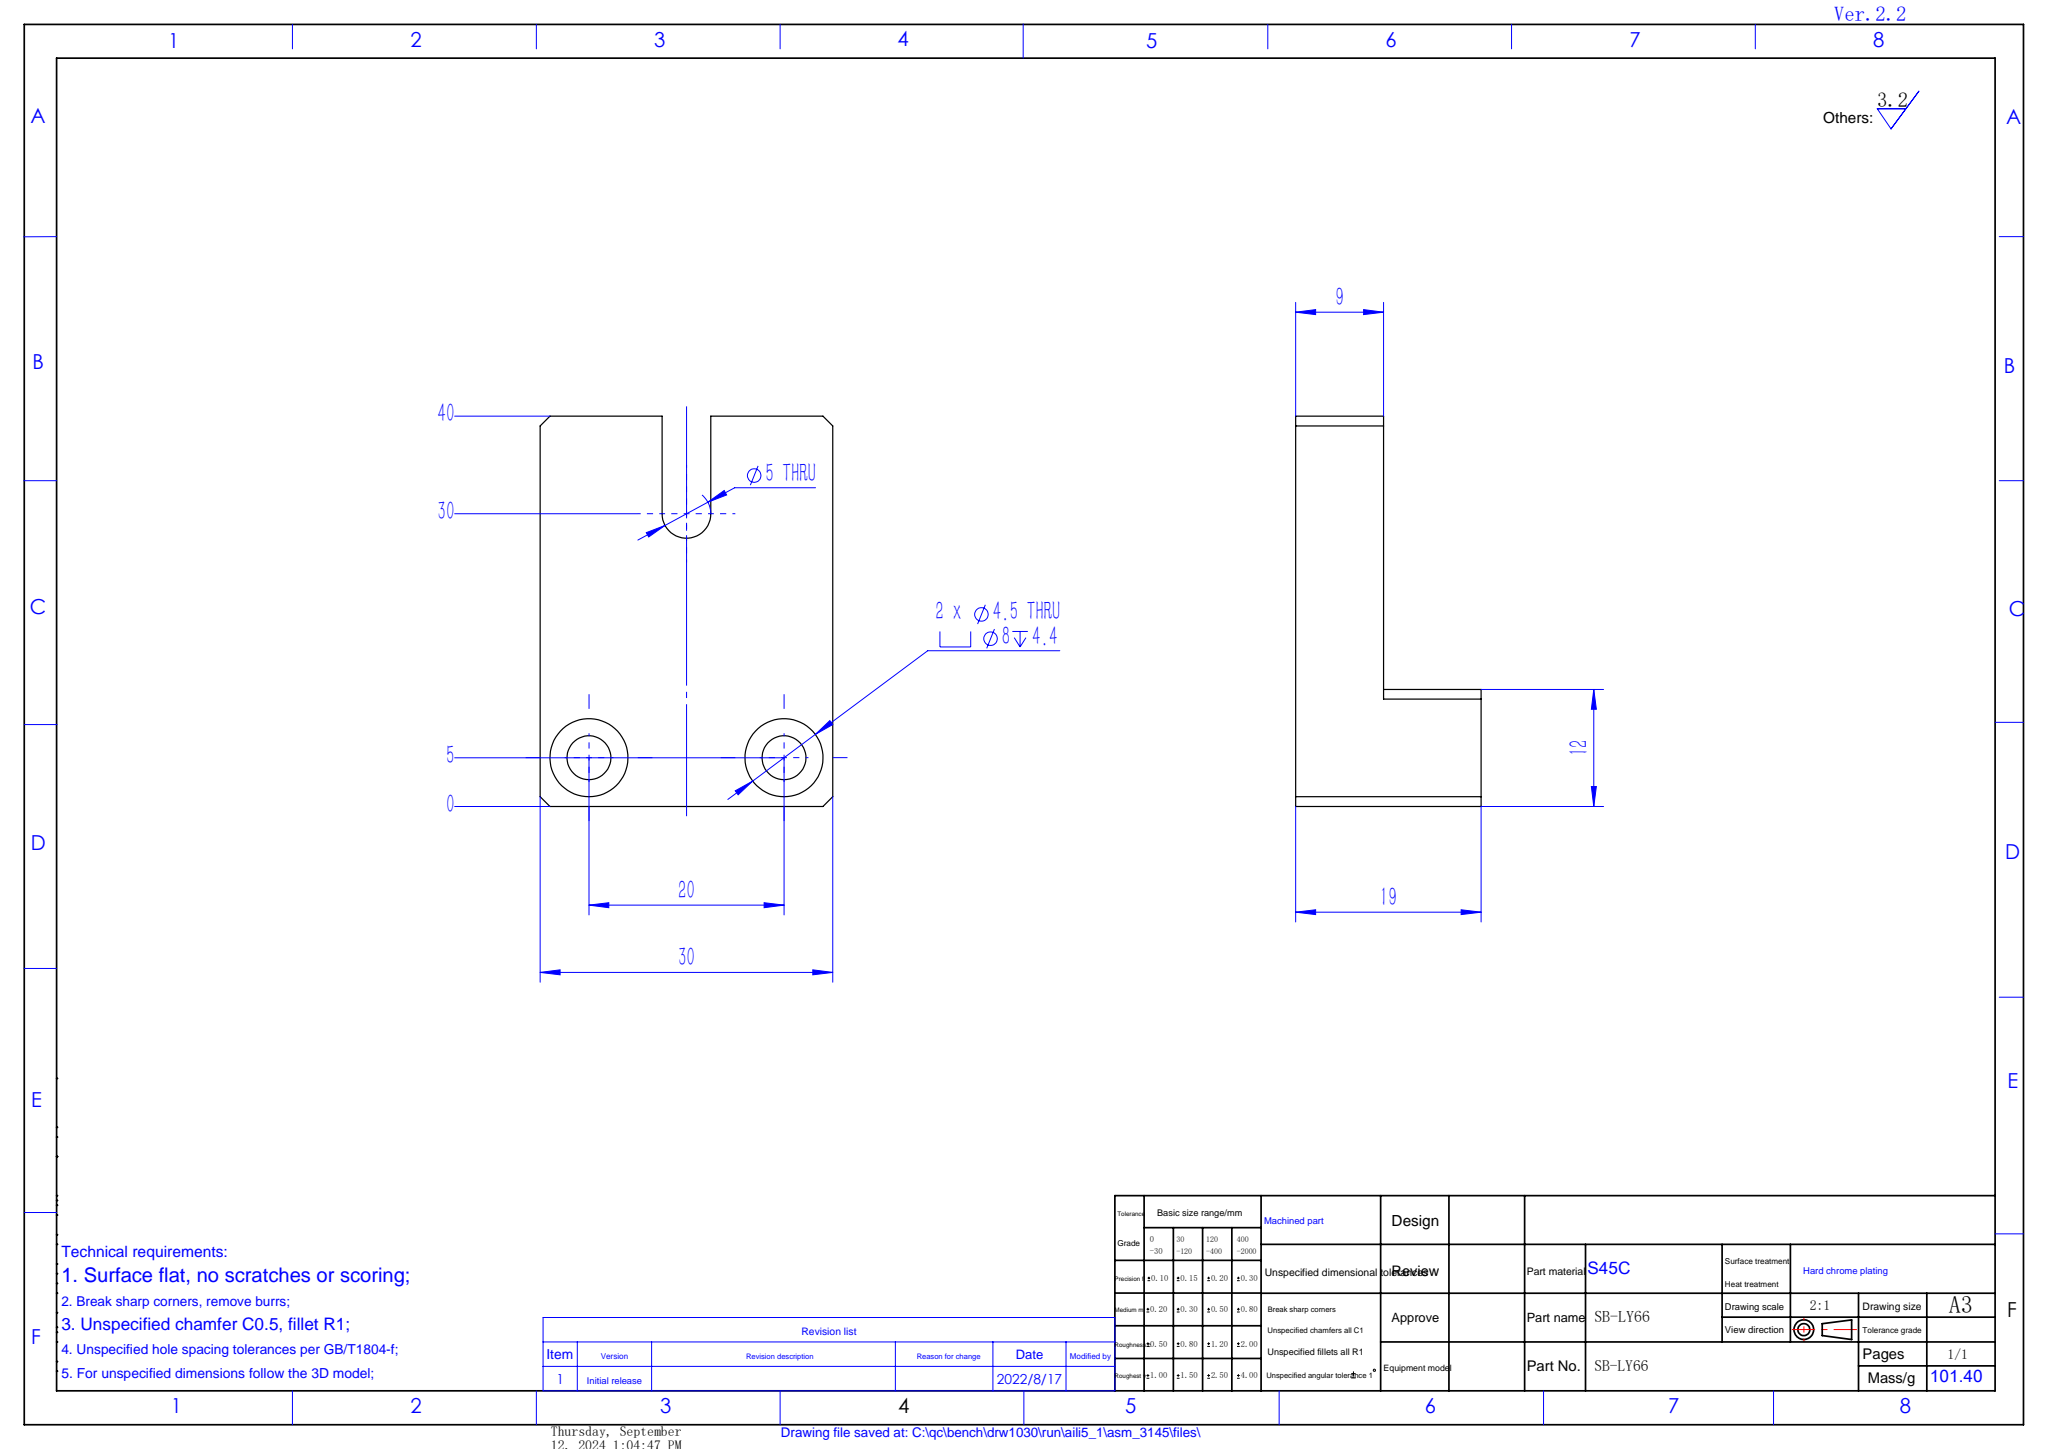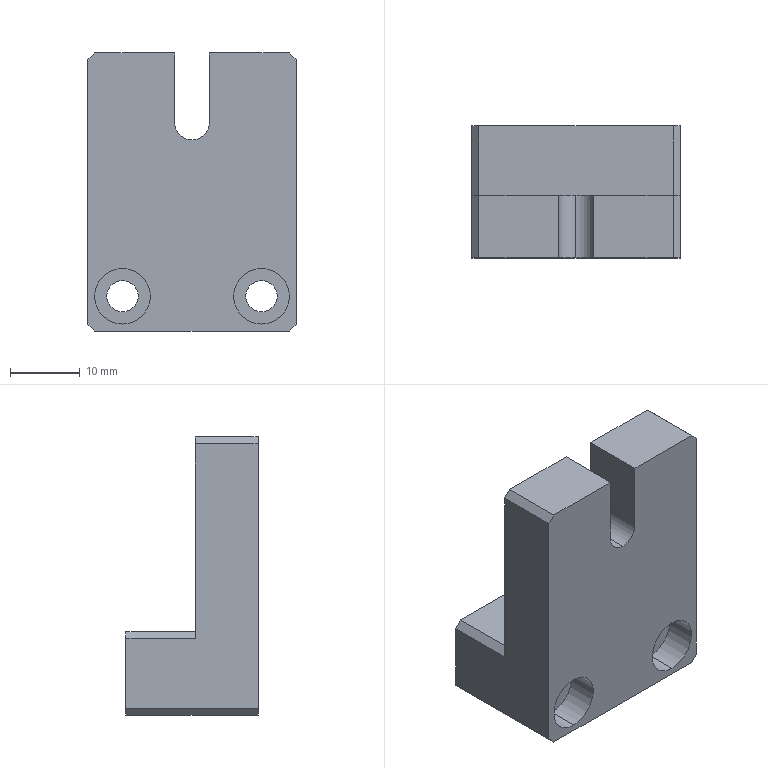Part | SolidWorks | features ICE 2, Chamfer 1, Extrusion 1, HoleWzd 1 | 1 solid | 29 faces | box 30 x 19 x 40 mm | volume 12917 mm3 | plane 19 | cylinder 10 | commonest cylinder face diameters 4.5 x4 8 x4 5 x2
STEP:
#1=CARTESIAN_POINT('',(2.5,9.,10.));
#2=VERTEX_POINT('',#1);
#3=CARTESIAN_POINT('',(0.,9.,7.5));
#4=VERTEX_POINT('',#3);
#5=CARTESIAN_POINT('',(0.,9.,10.));
#6=DIRECTION('',(0.,1.,0.));
#7=DIRECTION('',(0.,0.,1.));
#8=AXIS2_PLACEMENT_3D('',#5,#6,#7);
#9=CIRCLE('',#8,2.5);
#10=EDGE_CURVE('',#2,#4,#9,.T.);
#11=ORIENTED_EDGE('',*,*,#10,.T.);
#12=CARTESIAN_POINT('',(0.,0.,7.5));
#13=VERTEX_POINT('',#12);
#14=CARTESIAN_POINT('',(0.,19.,7.5));
#15=DIRECTION('',(0.,-1.,0.));
#16=VECTOR('',#15,1000.);
#17=LINE('',#14,#16);
#18=EDGE_CURVE('',#4,#13,#17,.T.);
#19=ORIENTED_EDGE('',*,*,#18,.T.);
#20=CARTESIAN_POINT('',(2.5,0.,10.));
#21=VERTEX_POINT('',#20);
#22=CARTESIAN_POINT('',(0.,0.,10.));
#23=DIRECTION('',(0.,-1.,0.));
#24=DIRECTION('',(0.,0.,-1.));
#25=AXIS2_PLACEMENT_3D('',#22,#23,#24);
#26=CIRCLE('',#25,2.5);
#27=EDGE_CURVE('',#13,#21,#26,.T.);
#28=ORIENTED_EDGE('',*,*,#27,.T.);
#29=CARTESIAN_POINT('',(2.5,19.,10.));
#30=DIRECTION('',(0.,-1.,0.));
#31=VECTOR('',#30,1000.);
#32=LINE('',#29,#31);
#33=EDGE_CURVE('',#2,#21,#32,.T.);
#34=ORIENTED_EDGE('',*,*,#33,.F.);
#35=EDGE_LOOP('',(#11,#19,#28,#34));
#36=FACE_OUTER_BOUND('',#35,.T.);
#37=CARTESIAN_POINT('',(0.,19.,10.));
#38=DIRECTION('',(0.,-1.,0.));
#39=DIRECTION('',(0.,0.,-1.));
#40=AXIS2_PLACEMENT_3D('',#37,#38,#39);
#41=CYLINDRICAL_SURFACE('',#40,2.5);
#42=ADVANCED_FACE('',(#36),#41,.F.);
#43=CARTESIAN_POINT('',(10.,4.4,-11.));
#44=VERTEX_POINT('',#43);
#45=CARTESIAN_POINT('',(10.,4.4,-19.));
#46=VERTEX_POINT('',#45);
#47=CARTESIAN_POINT('',(10.,4.4,-15.));
#48=DIRECTION('',(0.,-1.,0.));
#49=DIRECTION('',(0.,0.,-1.));
#50=AXIS2_PLACEMENT_3D('',#47,#48,#49);
#51=CIRCLE('',#50,4.);
#52=EDGE_CURVE('',#44,#46,#51,.T.);
#53=ORIENTED_EDGE('',*,*,#52,.F.);
#54=CARTESIAN_POINT('',(10.,0.,-11.));
#55=VERTEX_POINT('',#54);
#56=CARTESIAN_POINT('',(10.,0.,-11.));
#57=DIRECTION('',(0.,-1.,0.));
#58=VECTOR('',#57,1000.);
#59=LINE('',#56,#58);
#60=EDGE_CURVE('',#44,#55,#59,.T.);
#61=ORIENTED_EDGE('',*,*,#60,.T.);
#62=CARTESIAN_POINT('',(10.,0.,-19.));
#63=VERTEX_POINT('',#62);
#64=CARTESIAN_POINT('',(10.,0.,-15.));
#65=DIRECTION('',(0.,-1.,0.));
#66=DIRECTION('',(0.,0.,-1.));
#67=AXIS2_PLACEMENT_3D('',#64,#65,#66);
#68=CIRCLE('',#67,4.);
#69=EDGE_CURVE('',#55,#63,#68,.T.);
#70=ORIENTED_EDGE('',*,*,#69,.T.);
#71=CARTESIAN_POINT('',(10.,0.,-19.));
#72=DIRECTION('',(0.,-1.,0.));
#73=VECTOR('',#72,1000.);
#74=LINE('',#71,#73);
#75=EDGE_CURVE('',#46,#63,#74,.T.);
#76=ORIENTED_EDGE('',*,*,#75,.F.);
#77=EDGE_LOOP('',(#53,#61,#70,#76));
#78=FACE_OUTER_BOUND('',#77,.T.);
#79=CARTESIAN_POINT('',(10.,0.,-15.));
#80=DIRECTION('',(0.,-1.,0.));
#81=DIRECTION('',(0.,0.,-1.));
#82=AXIS2_PLACEMENT_3D('',#79,#80,#81);
#83=CYLINDRICAL_SURFACE('',#82,4.);
#84=ADVANCED_FACE('',(#78),#83,.F.);
#85=CARTESIAN_POINT('',(10.,19.,-12.75));
#86=VERTEX_POINT('',#85);
#87=CARTESIAN_POINT('',(10.,19.,-17.25));
#88=VERTEX_POINT('',#87);
#89=CARTESIAN_POINT('',(10.,19.,-15.));
#90=DIRECTION('',(0.,-1.,0.));
#91=DIRECTION('',(0.,0.,-1.));
#92=AXIS2_PLACEMENT_3D('',#89,#90,#91);
#93=CIRCLE('',#92,2.25);
#94=EDGE_CURVE('',#86,#88,#93,.T.);
#95=ORIENTED_EDGE('',*,*,#94,.F.);
#96=CARTESIAN_POINT('',(10.,4.4,-12.75));
#97=VERTEX_POINT('',#96);
#98=CARTESIAN_POINT('',(10.,0.,-12.75));
#99=DIRECTION('',(0.,-1.,0.));
#100=VECTOR('',#99,1000.);
#101=LINE('',#98,#100);
#102=EDGE_CURVE('',#86,#97,#101,.T.);
#103=ORIENTED_EDGE('',*,*,#102,.T.);
#104=CARTESIAN_POINT('',(10.,4.4,-17.25));
#105=VERTEX_POINT('',#104);
#106=CARTESIAN_POINT('',(10.,4.4,-15.));
#107=DIRECTION('',(0.,-1.,0.));
#108=DIRECTION('',(0.,0.,-1.));
#109=AXIS2_PLACEMENT_3D('',#106,#107,#108);
#110=CIRCLE('',#109,2.25);
#111=EDGE_CURVE('',#97,#105,#110,.T.);
#112=ORIENTED_EDGE('',*,*,#111,.T.);
#113=CARTESIAN_POINT('',(10.,0.,-17.25));
#114=DIRECTION('',(0.,-1.,0.));
#115=VECTOR('',#114,1000.);
#116=LINE('',#113,#115);
#117=EDGE_CURVE('',#88,#105,#116,.T.);
#118=ORIENTED_EDGE('',*,*,#117,.F.);
#119=EDGE_LOOP('',(#95,#103,#112,#118));
#120=FACE_OUTER_BOUND('',#119,.T.);
#121=CARTESIAN_POINT('',(10.,0.,-15.));
#122=DIRECTION('',(0.,-1.,0.));
#123=DIRECTION('',(0.,0.,-1.));
#124=AXIS2_PLACEMENT_3D('',#121,#122,#123);
#125=CYLINDRICAL_SURFACE('',#124,2.25);
#126=ADVANCED_FACE('',(#120),#125,.F.);
#127=CARTESIAN_POINT('',(-10.,4.4,-11.));
#128=VERTEX_POINT('',#127);
#129=CARTESIAN_POINT('',(-10.,4.4,-19.));
#130=VERTEX_POINT('',#129);
#131=CARTESIAN_POINT('',(-10.,4.4,-15.));
#132=DIRECTION('',(0.,-1.,0.));
#133=DIRECTION('',(0.,0.,-1.));
#134=AXIS2_PLACEMENT_3D('',#131,#132,#133);
#135=CIRCLE('',#134,4.);
#136=EDGE_CURVE('',#128,#130,#135,.T.);
#137=ORIENTED_EDGE('',*,*,#136,.F.);
#138=CARTESIAN_POINT('',(-10.,0.,-11.));
#139=VERTEX_POINT('',#138);
#140=CARTESIAN_POINT('',(-10.,0.,-11.));
#141=DIRECTION('',(0.,-1.,0.));
#142=VECTOR('',#141,1000.);
#143=LINE('',#140,#142);
#144=EDGE_CURVE('',#128,#139,#143,.T.);
#145=ORIENTED_EDGE('',*,*,#144,.T.);
#146=CARTESIAN_POINT('',(-10.,0.,-19.));
#147=VERTEX_POINT('',#146);
#148=CARTESIAN_POINT('',(-10.,0.,-15.));
#149=DIRECTION('',(0.,-1.,0.));
#150=DIRECTION('',(0.,0.,-1.));
#151=AXIS2_PLACEMENT_3D('',#148,#149,#150);
#152=CIRCLE('',#151,4.);
#153=EDGE_CURVE('',#139,#147,#152,.T.);
#154=ORIENTED_EDGE('',*,*,#153,.T.);
#155=CARTESIAN_POINT('',(-10.,0.,-19.));
#156=DIRECTION('',(0.,-1.,0.));
#157=VECTOR('',#156,1000.);
#158=LINE('',#155,#157);
#159=EDGE_CURVE('',#130,#147,#158,.T.);
#160=ORIENTED_EDGE('',*,*,#159,.F.);
#161=EDGE_LOOP('',(#137,#145,#154,#160));
#162=FACE_OUTER_BOUND('',#161,.T.);
#163=CARTESIAN_POINT('',(-10.,0.,-15.));
#164=DIRECTION('',(0.,-1.,0.));
#165=DIRECTION('',(0.,0.,-1.));
#166=AXIS2_PLACEMENT_3D('',#163,#164,#165);
#167=CYLINDRICAL_SURFACE('',#166,4.);
#168=ADVANCED_FACE('',(#162),#167,.F.);
#169=CARTESIAN_POINT('',(-10.,19.,-12.75));
#170=VERTEX_POINT('',#169);
#171=CARTESIAN_POINT('',(-10.,19.,-17.25));
#172=VERTEX_POINT('',#171);
#173=CARTESIAN_POINT('',(-10.,19.,-15.));
#174=DIRECTION('',(0.,-1.,0.));
#175=DIRECTION('',(0.,0.,-1.));
#176=AXIS2_PLACEMENT_3D('',#173,#174,#175);
#177=CIRCLE('',#176,2.25);
#178=EDGE_CURVE('',#170,#172,#177,.T.);
#179=ORIENTED_EDGE('',*,*,#178,.F.);
#180=CARTESIAN_POINT('',(-10.,4.4,-12.75));
#181=VERTEX_POINT('',#180);
#182=CARTESIAN_POINT('',(-10.,0.,-12.75));
#183=DIRECTION('',(0.,-1.,0.));
#184=VECTOR('',#183,1000.);
#185=LINE('',#182,#184);
#186=EDGE_CURVE('',#170,#181,#185,.T.);
#187=ORIENTED_EDGE('',*,*,#186,.T.);
#188=CARTESIAN_POINT('',(-10.,4.4,-17.25));
#189=VERTEX_POINT('',#188);
#190=CARTESIAN_POINT('',(-10.,4.4,-15.));
#191=DIRECTION('',(0.,-1.,0.));
#192=DIRECTION('',(0.,0.,-1.));
#193=AXIS2_PLACEMENT_3D('',#190,#191,#192);
#194=CIRCLE('',#193,2.25);
#195=EDGE_CURVE('',#181,#189,#194,.T.);
#196=ORIENTED_EDGE('',*,*,#195,.T.);
#197=CARTESIAN_POINT('',(-10.,0.,-17.25));
#198=DIRECTION('',(0.,-1.,0.));
#199=VECTOR('',#198,1000.);
#200=LINE('',#197,#199);
#201=EDGE_CURVE('',#172,#189,#200,.T.);
#202=ORIENTED_EDGE('',*,*,#201,.F.);
#203=EDGE_LOOP('',(#179,#187,#196,#202));
#204=FACE_OUTER_BOUND('',#203,.T.);
#205=CARTESIAN_POINT('',(-10.,0.,-15.));
#206=DIRECTION('',(0.,-1.,0.));
#207=DIRECTION('',(0.,0.,-1.));
#208=AXIS2_PLACEMENT_3D('',#205,#206,#207);
#209=CYLINDRICAL_SURFACE('',#208,2.25);
#210=ADVANCED_FACE('',(#204),#209,.F.);
#211=CARTESIAN_POINT('',(2.5,9.,20.));
#212=VERTEX_POINT('',#211);
#213=CARTESIAN_POINT('',(14.,9.,20.));
#214=VERTEX_POINT('',#213);
#215=CARTESIAN_POINT('',(15.,9.,20.));
#216=DIRECTION('',(1.,0.,0.));
#217=VECTOR('',#216,1000.);
#218=LINE('',#215,#217);
#219=EDGE_CURVE('',#212,#214,#218,.T.);
#220=ORIENTED_EDGE('',*,*,#219,.F.);
#221=CARTESIAN_POINT('',(2.5,0.,20.));
#222=VERTEX_POINT('',#221);
#223=CARTESIAN_POINT('',(2.5,19.,20.));
#224=DIRECTION('',(0.,-1.,0.));
#225=VECTOR('',#224,1000.);
#226=LINE('',#223,#225);
#227=EDGE_CURVE('',#212,#222,#226,.T.);
#228=ORIENTED_EDGE('',*,*,#227,.T.);
#229=CARTESIAN_POINT('',(14.,0.,20.));
#230=VERTEX_POINT('',#229);
#231=CARTESIAN_POINT('',(15.,0.,20.));
#232=DIRECTION('',(1.,0.,0.));
#233=VECTOR('',#232,1000.);
#234=LINE('',#231,#233);
#235=EDGE_CURVE('',#222,#230,#234,.T.);
#236=ORIENTED_EDGE('',*,*,#235,.T.);
#237=CARTESIAN_POINT('',(14.,9.,20.));
#238=DIRECTION('',(0.,1.,0.));
#239=VECTOR('',#238,1000.);
#240=LINE('',#237,#239);
#241=EDGE_CURVE('',#230,#214,#240,.T.);
#242=ORIENTED_EDGE('',*,*,#241,.T.);
#243=EDGE_LOOP('',(#220,#228,#236,#242));
#244=FACE_OUTER_BOUND('',#243,.T.);
#245=CARTESIAN_POINT('',(15.,9.,20.));
#246=DIRECTION('',(0.,0.,-1.));
#247=DIRECTION('',(-1.,0.,0.));
#248=AXIS2_PLACEMENT_3D('',#245,#246,#247);
#249=PLANE('',#248);
#250=ADVANCED_FACE('',(#244),#249,.F.);
#251=CARTESIAN_POINT('',(-15.,0.,-19.));
#252=VERTEX_POINT('',#251);
#253=CARTESIAN_POINT('',(-15.,0.,19.));
#254=VERTEX_POINT('',#253);
#255=CARTESIAN_POINT('',(-15.,0.,20.));
#256=DIRECTION('',(0.,0.,1.));
#257=VECTOR('',#256,1000.);
#258=LINE('',#255,#257);
#259=EDGE_CURVE('',#252,#254,#258,.T.);
#260=ORIENTED_EDGE('',*,*,#259,.T.);
#261=CARTESIAN_POINT('',(-15.,9.,19.));
#262=VERTEX_POINT('',#261);
#263=CARTESIAN_POINT('',(-15.,9.,19.));
#264=DIRECTION('',(0.,1.,0.));
#265=VECTOR('',#264,1000.);
#266=LINE('',#263,#265);
#267=EDGE_CURVE('',#254,#262,#266,.T.);
#268=ORIENTED_EDGE('',*,*,#267,.T.);
#269=CARTESIAN_POINT('',(-15.,9.,-9.));
#270=VERTEX_POINT('',#269);
#271=CARTESIAN_POINT('',(-15.,9.,20.));
#272=DIRECTION('',(0.,0.,1.));
#273=VECTOR('',#272,1000.);
#274=LINE('',#271,#273);
#275=EDGE_CURVE('',#270,#262,#274,.T.);
#276=ORIENTED_EDGE('',*,*,#275,.F.);
#277=CARTESIAN_POINT('',(-15.,19.,-9.));
#278=VERTEX_POINT('',#277);
#279=CARTESIAN_POINT('',(-15.,9.,-9.));
#280=DIRECTION('',(0.,1.,0.));
#281=VECTOR('',#280,1000.);
#282=LINE('',#279,#281);
#283=EDGE_CURVE('',#270,#278,#282,.T.);
#284=ORIENTED_EDGE('',*,*,#283,.T.);
#285=CARTESIAN_POINT('',(-15.,19.,-19.));
#286=VERTEX_POINT('',#285);
#287=CARTESIAN_POINT('',(-15.,19.,-20.));
#288=DIRECTION('',(0.,0.,1.));
#289=VECTOR('',#288,1000.);
#290=LINE('',#287,#289);
#291=EDGE_CURVE('',#286,#278,#290,.T.);
#292=ORIENTED_EDGE('',*,*,#291,.F.);
#293=CARTESIAN_POINT('',(-15.,9.,-19.));
#294=DIRECTION('',(0.,-1.,0.));
#295=VECTOR('',#294,1000.);
#296=LINE('',#293,#295);
#297=EDGE_CURVE('',#286,#252,#296,.T.);
#298=ORIENTED_EDGE('',*,*,#297,.T.);
#299=EDGE_LOOP('',(#260,#268,#276,#284,#292,#298));
#300=FACE_OUTER_BOUND('',#299,.T.);
#301=CARTESIAN_POINT('',(-15.,9.,20.));
#302=DIRECTION('',(1.,0.,0.));
#303=DIRECTION('',(0.,0.,-1.));
#304=AXIS2_PLACEMENT_3D('',#301,#302,#303);
#305=PLANE('',#304);
#306=ADVANCED_FACE('',(#300),#305,.F.);
#307=CARTESIAN_POINT('',(-14.,0.,20.));
#308=VERTEX_POINT('',#307);
#309=CARTESIAN_POINT('',(-2.5,0.,20.));
#310=VERTEX_POINT('',#309);
#311=CARTESIAN_POINT('',(15.,0.,20.));
#312=DIRECTION('',(1.,0.,0.));
#313=VECTOR('',#312,1000.);
#314=LINE('',#311,#313);
#315=EDGE_CURVE('',#308,#310,#314,.T.);
#316=ORIENTED_EDGE('',*,*,#315,.T.);
#317=CARTESIAN_POINT('',(-2.5,9.,20.));
#318=VERTEX_POINT('',#317);
#319=CARTESIAN_POINT('',(-2.5,19.,20.));
#320=DIRECTION('',(0.,-1.,0.));
#321=VECTOR('',#320,1000.);
#322=LINE('',#319,#321);
#323=EDGE_CURVE('',#318,#310,#322,.T.);
#324=ORIENTED_EDGE('',*,*,#323,.F.);
#325=CARTESIAN_POINT('',(-14.,9.,20.));
#326=VERTEX_POINT('',#325);
#327=CARTESIAN_POINT('',(15.,9.,20.));
#328=DIRECTION('',(1.,0.,0.));
#329=VECTOR('',#328,1000.);
#330=LINE('',#327,#329);
#331=EDGE_CURVE('',#326,#318,#330,.T.);
#332=ORIENTED_EDGE('',*,*,#331,.F.);
#333=CARTESIAN_POINT('',(-14.,9.,20.));
#334=DIRECTION('',(0.,-1.,0.));
#335=VECTOR('',#334,1000.);
#336=LINE('',#333,#335);
#337=EDGE_CURVE('',#326,#308,#336,.T.);
#338=ORIENTED_EDGE('',*,*,#337,.T.);
#339=EDGE_LOOP('',(#316,#324,#332,#338));
#340=FACE_OUTER_BOUND('',#339,.T.);
#341=CARTESIAN_POINT('',(15.,9.,20.));
#342=DIRECTION('',(0.,0.,-1.));
#343=DIRECTION('',(-1.,0.,0.));
#344=AXIS2_PLACEMENT_3D('',#341,#342,#343);
#345=PLANE('',#344);
#346=ADVANCED_FACE('',(#340),#345,.F.);
#347=CARTESIAN_POINT('',(15.,9.,19.));
#348=VERTEX_POINT('',#347);
#349=CARTESIAN_POINT('',(15.,9.,-9.));
#350=VERTEX_POINT('',#349);
#351=CARTESIAN_POINT('',(15.,9.,20.));
#352=DIRECTION('',(0.,0.,-1.));
#353=VECTOR('',#352,1000.);
#354=LINE('',#351,#353);
#355=EDGE_CURVE('',#348,#350,#354,.T.);
#356=ORIENTED_EDGE('',*,*,#355,.F.);
#357=CARTESIAN_POINT('',(15.,0.,19.));
#358=VERTEX_POINT('',#357);
#359=CARTESIAN_POINT('',(15.,9.,19.));
#360=DIRECTION('',(0.,-1.,0.));
#361=VECTOR('',#360,1000.);
#362=LINE('',#359,#361);
#363=EDGE_CURVE('',#348,#358,#362,.T.);
#364=ORIENTED_EDGE('',*,*,#363,.T.);
#365=CARTESIAN_POINT('',(15.,0.,-19.));
#366=VERTEX_POINT('',#365);
#367=CARTESIAN_POINT('',(15.,0.,20.));
#368=DIRECTION('',(0.,0.,-1.));
#369=VECTOR('',#368,1000.);
#370=LINE('',#367,#369);
#371=EDGE_CURVE('',#358,#366,#370,.T.);
#372=ORIENTED_EDGE('',*,*,#371,.T.);
#373=CARTESIAN_POINT('',(15.,19.,-19.));
#374=VERTEX_POINT('',#373);
#375=CARTESIAN_POINT('',(15.,9.,-19.));
#376=DIRECTION('',(0.,1.,0.));
#377=VECTOR('',#376,1000.);
#378=LINE('',#375,#377);
#379=EDGE_CURVE('',#366,#374,#378,.T.);
#380=ORIENTED_EDGE('',*,*,#379,.T.);
#381=CARTESIAN_POINT('',(15.,19.,-9.));
#382=VERTEX_POINT('',#381);
#383=CARTESIAN_POINT('',(15.,19.,-20.));
#384=DIRECTION('',(0.,0.,-1.));
#385=VECTOR('',#384,1000.);
#386=LINE('',#383,#385);
#387=EDGE_CURVE('',#382,#374,#386,.T.);
#388=ORIENTED_EDGE('',*,*,#387,.F.);
#389=CARTESIAN_POINT('',(15.,9.,-9.));
#390=DIRECTION('',(0.,-1.,0.));
#391=VECTOR('',#390,1000.);
#392=LINE('',#389,#391);
#393=EDGE_CURVE('',#382,#350,#392,.T.);
#394=ORIENTED_EDGE('',*,*,#393,.T.);
#395=EDGE_LOOP('',(#356,#364,#372,#380,#388,#394));
#396=FACE_OUTER_BOUND('',#395,.T.);
#397=CARTESIAN_POINT('',(15.,9.,20.));
#398=DIRECTION('',(-1.,0.,0.));
#399=DIRECTION('',(0.,0.,1.));
#400=AXIS2_PLACEMENT_3D('',#397,#398,#399);
#401=PLANE('',#400);
#402=ADVANCED_FACE('',(#396),#401,.F.);
#403=CARTESIAN_POINT('',(14.,0.,-20.));
#404=VERTEX_POINT('',#403);
#405=CARTESIAN_POINT('',(-14.,0.,-20.));
#406=VERTEX_POINT('',#405);
#407=CARTESIAN_POINT('',(15.,0.,-20.));
#408=DIRECTION('',(-1.,0.,0.));
#409=VECTOR('',#408,1000.);
#410=LINE('',#407,#409);
#411=EDGE_CURVE('',#404,#406,#410,.T.);
#412=ORIENTED_EDGE('',*,*,#411,.T.);
#413=CARTESIAN_POINT('',(-14.,19.,-20.));
#414=VERTEX_POINT('',#413);
#415=CARTESIAN_POINT('',(-14.,9.,-20.));
#416=DIRECTION('',(0.,1.,0.));
#417=VECTOR('',#416,1000.);
#418=LINE('',#415,#417);
#419=EDGE_CURVE('',#406,#414,#418,.T.);
#420=ORIENTED_EDGE('',*,*,#419,.T.);
#421=CARTESIAN_POINT('',(14.,19.,-20.));
#422=VERTEX_POINT('',#421);
#423=CARTESIAN_POINT('',(-15.,19.,-20.));
#424=DIRECTION('',(-1.,0.,0.));
#425=VECTOR('',#424,1000.);
#426=LINE('',#423,#425);
#427=EDGE_CURVE('',#422,#414,#426,.T.);
#428=ORIENTED_EDGE('',*,*,#427,.F.);
#429=CARTESIAN_POINT('',(14.,9.,-20.));
#430=DIRECTION('',(0.,-1.,0.));
#431=VECTOR('',#430,1000.);
#432=LINE('',#429,#431);
#433=EDGE_CURVE('',#422,#404,#432,.T.);
#434=ORIENTED_EDGE('',*,*,#433,.T.);
#435=EDGE_LOOP('',(#412,#420,#428,#434));
#436=FACE_OUTER_BOUND('',#435,.T.);
#437=CARTESIAN_POINT('',(15.,9.,-20.));
#438=DIRECTION('',(0.,0.,1.));
#439=DIRECTION('',(1.,0.,0.));
#440=AXIS2_PLACEMENT_3D('',#437,#438,#439);
#441=PLANE('',#440);
#442=ADVANCED_FACE('',(#436),#441,.F.);
#443=CARTESIAN_POINT('',(2.5,9.,0.));
#444=DIRECTION('',(0.,0.,-1.));
#445=VECTOR('',#444,1000.);
#446=LINE('',#443,#445);
#447=EDGE_CURVE('',#212,#2,#446,.T.);
#448=ORIENTED_EDGE('',*,*,#447,.F.);
#449=ORIENTED_EDGE('',*,*,#219,.T.);
#450=CARTESIAN_POINT('',(17.,9.,17.));
#451=DIRECTION('',(0.7071,0.,-0.7071));
#452=VECTOR('',#451,1000.);
#453=LINE('',#450,#452);
#454=EDGE_CURVE('',#214,#348,#453,.T.);
#455=ORIENTED_EDGE('',*,*,#454,.T.);
#456=ORIENTED_EDGE('',*,*,#355,.T.);
#457=CARTESIAN_POINT('',(14.,9.,-8.));
#458=VERTEX_POINT('',#457);
#459=CARTESIAN_POINT('',(15.,9.,-9.));
#460=DIRECTION('',(-0.7071,0.,0.7071));
#461=VECTOR('',#460,1000.);
#462=LINE('',#459,#461);
#463=EDGE_CURVE('',#350,#458,#462,.T.);
#464=ORIENTED_EDGE('',*,*,#463,.T.);
#465=CARTESIAN_POINT('',(-14.,9.,-8.));
#466=VERTEX_POINT('',#465);
#467=CARTESIAN_POINT('',(-15.,9.,-8.));
#468=DIRECTION('',(1.,0.,0.));
#469=VECTOR('',#468,1000.);
#470=LINE('',#467,#469);
#471=EDGE_CURVE('',#466,#458,#470,.T.);
#472=ORIENTED_EDGE('',*,*,#471,.F.);
#473=CARTESIAN_POINT('',(-14.,9.,-8.));
#474=DIRECTION('',(-0.7071,0.,-0.7071));
#475=VECTOR('',#474,1000.);
#476=LINE('',#473,#475);
#477=EDGE_CURVE('',#466,#270,#476,.T.);
#478=ORIENTED_EDGE('',*,*,#477,.T.);
#479=ORIENTED_EDGE('',*,*,#275,.T.);
#480=CARTESIAN_POINT('',(-17.,9.,17.));
#481=DIRECTION('',(0.7071,0.,0.7071));
#482=VECTOR('',#481,1000.);
#483=LINE('',#480,#482);
#484=EDGE_CURVE('',#262,#326,#483,.T.);
#485=ORIENTED_EDGE('',*,*,#484,.T.);
#486=ORIENTED_EDGE('',*,*,#331,.T.);
#487=CARTESIAN_POINT('',(-2.5,9.,10.));
#488=VERTEX_POINT('',#487);
#489=CARTESIAN_POINT('',(-2.5,9.,0.));
#490=DIRECTION('',(0.,0.,1.));
#491=VECTOR('',#490,1000.);
#492=LINE('',#489,#491);
#493=EDGE_CURVE('',#488,#318,#492,.T.);
#494=ORIENTED_EDGE('',*,*,#493,.F.);
#495=CARTESIAN_POINT('',(0.,9.,10.));
#496=DIRECTION('',(0.,1.,0.));
#497=DIRECTION('',(0.,0.,1.));
#498=AXIS2_PLACEMENT_3D('',#495,#496,#497);
#499=CIRCLE('',#498,2.5);
#500=EDGE_CURVE('',#4,#488,#499,.T.);
#501=ORIENTED_EDGE('',*,*,#500,.F.);
#502=ORIENTED_EDGE('',*,*,#10,.F.);
#503=EDGE_LOOP('',(#448,#449,#455,#456,#464,#472,#478,#479,#485,#486,#494,#501,#502));
#504=FACE_OUTER_BOUND('',#503,.T.);
#505=CARTESIAN_POINT('',(0.,9.,0.));
#506=DIRECTION('',(0.,1.,0.));
#507=DIRECTION('',(0.,0.,1.));
#508=AXIS2_PLACEMENT_3D('',#505,#506,#507);
#509=PLANE('',#508);
#510=ADVANCED_FACE('',(#504),#509,.T.);
#511=CARTESIAN_POINT('',(10.,0.,-15.));
#512=DIRECTION('',(0.,-1.,0.));
#513=DIRECTION('',(0.,0.,-1.));
#514=AXIS2_PLACEMENT_3D('',#511,#512,#513);
#515=CIRCLE('',#514,4.);
#516=EDGE_CURVE('',#63,#55,#515,.T.);
#517=ORIENTED_EDGE('',*,*,#516,.F.);
#518=ORIENTED_EDGE('',*,*,#69,.F.);
#519=EDGE_LOOP('',(#517,#518));
#520=FACE_BOUND('',#519,.T.);
#521=CARTESIAN_POINT('',(-10.,0.,-15.));
#522=DIRECTION('',(0.,-1.,0.));
#523=DIRECTION('',(0.,0.,-1.));
#524=AXIS2_PLACEMENT_3D('',#521,#522,#523);
#525=CIRCLE('',#524,4.);
#526=EDGE_CURVE('',#147,#139,#525,.T.);
#527=ORIENTED_EDGE('',*,*,#526,.F.);
#528=ORIENTED_EDGE('',*,*,#153,.F.);
#529=EDGE_LOOP('',(#527,#528));
#530=FACE_BOUND('',#529,.T.);
#531=ORIENTED_EDGE('',*,*,#235,.F.);
#532=CARTESIAN_POINT('',(2.5,0.,20.));
#533=DIRECTION('',(0.,0.,1.));
#534=VECTOR('',#533,1000.);
#535=LINE('',#532,#534);
#536=EDGE_CURVE('',#21,#222,#535,.T.);
#537=ORIENTED_EDGE('',*,*,#536,.F.);
#538=ORIENTED_EDGE('',*,*,#27,.F.);
#539=CARTESIAN_POINT('',(-2.5,0.,10.));
#540=VERTEX_POINT('',#539);
#541=CARTESIAN_POINT('',(0.,0.,10.));
#542=DIRECTION('',(0.,-1.,0.));
#543=DIRECTION('',(0.,0.,-1.));
#544=AXIS2_PLACEMENT_3D('',#541,#542,#543);
#545=CIRCLE('',#544,2.5);
#546=EDGE_CURVE('',#540,#13,#545,.T.);
#547=ORIENTED_EDGE('',*,*,#546,.F.);
#548=CARTESIAN_POINT('',(-2.5,0.,20.));
#549=DIRECTION('',(0.,0.,-1.));
#550=VECTOR('',#549,1000.);
#551=LINE('',#548,#550);
#552=EDGE_CURVE('',#310,#540,#551,.T.);
#553=ORIENTED_EDGE('',*,*,#552,.F.);
#554=ORIENTED_EDGE('',*,*,#315,.F.);
#555=CARTESIAN_POINT('',(-14.,0.,20.));
#556=DIRECTION('',(-0.7071,0.,-0.7071));
#557=VECTOR('',#556,1000.);
#558=LINE('',#555,#557);
#559=EDGE_CURVE('',#308,#254,#558,.T.);
#560=ORIENTED_EDGE('',*,*,#559,.T.);
#561=ORIENTED_EDGE('',*,*,#259,.F.);
#562=CARTESIAN_POINT('',(-15.,0.,-19.));
#563=DIRECTION('',(0.7071,0.,-0.7071));
#564=VECTOR('',#563,1000.);
#565=LINE('',#562,#564);
#566=EDGE_CURVE('',#252,#406,#565,.T.);
#567=ORIENTED_EDGE('',*,*,#566,.T.);
#568=ORIENTED_EDGE('',*,*,#411,.F.);
#569=CARTESIAN_POINT('',(14.,0.,-20.));
#570=DIRECTION('',(0.7071,0.,0.7071));
#571=VECTOR('',#570,1000.);
#572=LINE('',#569,#571);
#573=EDGE_CURVE('',#404,#366,#572,.T.);
#574=ORIENTED_EDGE('',*,*,#573,.T.);
#575=ORIENTED_EDGE('',*,*,#371,.F.);
#576=CARTESIAN_POINT('',(15.,0.,19.));
#577=DIRECTION('',(-0.7071,0.,0.7071));
#578=VECTOR('',#577,1000.);
#579=LINE('',#576,#578);
#580=EDGE_CURVE('',#358,#230,#579,.T.);
#581=ORIENTED_EDGE('',*,*,#580,.T.);
#582=EDGE_LOOP('',(#531,#537,#538,#547,#553,#554,#560,#561,#567,#568,#574,#575,#581));
#583=FACE_OUTER_BOUND('',#582,.T.);
#584=CARTESIAN_POINT('',(0.,0.,0.));
#585=DIRECTION('',(0.,1.,0.));
#586=DIRECTION('',(0.,0.,1.));
#587=AXIS2_PLACEMENT_3D('',#584,#585,#586);
#588=PLANE('',#587);
#589=ADVANCED_FACE('',(#520,#530,#583),#588,.F.);
#590=CARTESIAN_POINT('',(-14.,19.,-8.));
#591=VERTEX_POINT('',#590);
#592=CARTESIAN_POINT('',(14.,19.,-8.));
#593=VERTEX_POINT('',#592);
#594=CARTESIAN_POINT('',(-15.,19.,-8.));
#595=DIRECTION('',(1.,0.,0.));
#596=VECTOR('',#595,1000.);
#597=LINE('',#594,#596);
#598=EDGE_CURVE('',#591,#593,#597,.T.);
#599=ORIENTED_EDGE('',*,*,#598,.F.);
#600=CARTESIAN_POINT('',(-14.,19.,-8.));
#601=DIRECTION('',(0.,-1.,0.));
#602=VECTOR('',#601,1000.);
#603=LINE('',#600,#602);
#604=EDGE_CURVE('',#591,#466,#603,.T.);
#605=ORIENTED_EDGE('',*,*,#604,.T.);
#606=ORIENTED_EDGE('',*,*,#471,.T.);
#607=CARTESIAN_POINT('',(14.,19.,-8.));
#608=DIRECTION('',(0.,1.,0.));
#609=VECTOR('',#608,1000.);
#610=LINE('',#607,#609);
#611=EDGE_CURVE('',#458,#593,#610,.T.);
#612=ORIENTED_EDGE('',*,*,#611,.T.);
#613=EDGE_LOOP('',(#599,#605,#606,#612));
#614=FACE_OUTER_BOUND('',#613,.T.);
#615=CARTESIAN_POINT('',(-15.,19.,-8.));
#616=DIRECTION('',(0.,0.,-1.));
#617=DIRECTION('',(-1.,0.,0.));
#618=AXIS2_PLACEMENT_3D('',#615,#616,#617);
#619=PLANE('',#618);
#620=ADVANCED_FACE('',(#614),#619,.F.);
#621=CARTESIAN_POINT('',(10.,19.,-15.));
#622=DIRECTION('',(0.,-1.,0.));
#623=DIRECTION('',(0.,0.,-1.));
#624=AXIS2_PLACEMENT_3D('',#621,#622,#623);
#625=CIRCLE('',#624,2.25);
#626=EDGE_CURVE('',#88,#86,#625,.T.);
#627=ORIENTED_EDGE('',*,*,#626,.T.);
#628=ORIENTED_EDGE('',*,*,#94,.T.);
#629=EDGE_LOOP('',(#627,#628));
#630=FACE_BOUND('',#629,.T.);
#631=CARTESIAN_POINT('',(-10.,19.,-15.));
#632=DIRECTION('',(0.,-1.,0.));
#633=DIRECTION('',(0.,0.,-1.));
#634=AXIS2_PLACEMENT_3D('',#631,#632,#633);
#635=CIRCLE('',#634,2.25);
#636=EDGE_CURVE('',#172,#170,#635,.T.);
#637=ORIENTED_EDGE('',*,*,#636,.T.);
#638=ORIENTED_EDGE('',*,*,#178,.T.);
#639=EDGE_LOOP('',(#637,#638));
#640=FACE_BOUND('',#639,.T.);
#641=ORIENTED_EDGE('',*,*,#291,.T.);
#642=CARTESIAN_POINT('',(-3.,19.,3.));
#643=DIRECTION('',(0.7071,0.,0.7071));
#644=VECTOR('',#643,1000.);
#645=LINE('',#642,#644);
#646=EDGE_CURVE('',#278,#591,#645,.T.);
#647=ORIENTED_EDGE('',*,*,#646,.T.);
#648=ORIENTED_EDGE('',*,*,#598,.T.);
#649=CARTESIAN_POINT('',(3.,19.,3.));
#650=DIRECTION('',(0.7071,0.,-0.7071));
#651=VECTOR('',#650,1000.);
#652=LINE('',#649,#651);
#653=EDGE_CURVE('',#593,#382,#652,.T.);
#654=ORIENTED_EDGE('',*,*,#653,.T.);
#655=ORIENTED_EDGE('',*,*,#387,.T.);
#656=CARTESIAN_POINT('',(17.,19.,-17.));
#657=DIRECTION('',(-0.7071,0.,-0.7071));
#658=VECTOR('',#657,1000.);
#659=LINE('',#656,#658);
#660=EDGE_CURVE('',#374,#422,#659,.T.);
#661=ORIENTED_EDGE('',*,*,#660,.T.);
#662=ORIENTED_EDGE('',*,*,#427,.T.);
#663=CARTESIAN_POINT('',(-17.,19.,-17.));
#664=DIRECTION('',(-0.7071,0.,0.7071));
#665=VECTOR('',#664,1000.);
#666=LINE('',#663,#665);
#667=EDGE_CURVE('',#414,#286,#666,.T.);
#668=ORIENTED_EDGE('',*,*,#667,.T.);
#669=EDGE_LOOP('',(#641,#647,#648,#654,#655,#661,#662,#668));
#670=FACE_OUTER_BOUND('',#669,.T.);
#671=CARTESIAN_POINT('',(0.,19.,0.));
#672=DIRECTION('',(0.,1.,0.));
#673=DIRECTION('',(0.,0.,1.));
#674=AXIS2_PLACEMENT_3D('',#671,#672,#673);
#675=PLANE('',#674);
#676=ADVANCED_FACE('',(#630,#640,#670),#675,.T.);
#677=ORIENTED_EDGE('',*,*,#186,.F.);
#678=ORIENTED_EDGE('',*,*,#636,.F.);
#679=ORIENTED_EDGE('',*,*,#201,.T.);
#680=CARTESIAN_POINT('',(-10.,4.4,-15.));
#681=DIRECTION('',(0.,-1.,0.));
#682=DIRECTION('',(0.,0.,-1.));
#683=AXIS2_PLACEMENT_3D('',#680,#681,#682);
#684=CIRCLE('',#683,2.25);
#685=EDGE_CURVE('',#189,#181,#684,.T.);
#686=ORIENTED_EDGE('',*,*,#685,.T.);
#687=EDGE_LOOP('',(#677,#678,#679,#686));
#688=FACE_OUTER_BOUND('',#687,.T.);
#689=CARTESIAN_POINT('',(-10.,0.,-15.));
#690=DIRECTION('',(0.,-1.,0.));
#691=DIRECTION('',(0.,0.,-1.));
#692=AXIS2_PLACEMENT_3D('',#689,#690,#691);
#693=CYLINDRICAL_SURFACE('',#692,2.25);
#694=ADVANCED_FACE('',(#688),#693,.F.);
#695=ORIENTED_EDGE('',*,*,#685,.F.);
#696=ORIENTED_EDGE('',*,*,#195,.F.);
#697=EDGE_LOOP('',(#695,#696));
#698=FACE_BOUND('',#697,.T.);
#699=CARTESIAN_POINT('',(-10.,4.4,-15.));
#700=DIRECTION('',(0.,-1.,0.));
#701=DIRECTION('',(0.,0.,-1.));
#702=AXIS2_PLACEMENT_3D('',#699,#700,#701);
#703=CIRCLE('',#702,4.);
#704=EDGE_CURVE('',#130,#128,#703,.T.);
#705=ORIENTED_EDGE('',*,*,#704,.T.);
#706=ORIENTED_EDGE('',*,*,#136,.T.);
#707=EDGE_LOOP('',(#705,#706));
#708=FACE_OUTER_BOUND('',#707,.T.);
#709=CARTESIAN_POINT('',(-7.75,4.4,-15.));
#710=DIRECTION('',(0.,1.,0.));
#711=DIRECTION('',(0.,0.,1.));
#712=AXIS2_PLACEMENT_3D('',#709,#710,#711);
#713=PLANE('',#712);
#714=ADVANCED_FACE('',(#698,#708),#713,.F.);
#715=ORIENTED_EDGE('',*,*,#144,.F.);
#716=ORIENTED_EDGE('',*,*,#704,.F.);
#717=ORIENTED_EDGE('',*,*,#159,.T.);
#718=ORIENTED_EDGE('',*,*,#526,.T.);
#719=EDGE_LOOP('',(#715,#716,#717,#718));
#720=FACE_OUTER_BOUND('',#719,.T.);
#721=CARTESIAN_POINT('',(-10.,0.,-15.));
#722=DIRECTION('',(0.,-1.,0.));
#723=DIRECTION('',(0.,0.,-1.));
#724=AXIS2_PLACEMENT_3D('',#721,#722,#723);
#725=CYLINDRICAL_SURFACE('',#724,4.);
#726=ADVANCED_FACE('',(#720),#725,.F.);
#727=ORIENTED_EDGE('',*,*,#102,.F.);
#728=ORIENTED_EDGE('',*,*,#626,.F.);
#729=ORIENTED_EDGE('',*,*,#117,.T.);
#730=CARTESIAN_POINT('',(10.,4.4,-15.));
#731=DIRECTION('',(0.,-1.,0.));
#732=DIRECTION('',(0.,0.,-1.));
#733=AXIS2_PLACEMENT_3D('',#730,#731,#732);
#734=CIRCLE('',#733,2.25);
#735=EDGE_CURVE('',#105,#97,#734,.T.);
#736=ORIENTED_EDGE('',*,*,#735,.T.);
#737=EDGE_LOOP('',(#727,#728,#729,#736));
#738=FACE_OUTER_BOUND('',#737,.T.);
#739=CARTESIAN_POINT('',(10.,0.,-15.));
#740=DIRECTION('',(0.,-1.,0.));
#741=DIRECTION('',(0.,0.,-1.));
#742=AXIS2_PLACEMENT_3D('',#739,#740,#741);
#743=CYLINDRICAL_SURFACE('',#742,2.25);
#744=ADVANCED_FACE('',(#738),#743,.F.);
#745=ORIENTED_EDGE('',*,*,#735,.F.);
#746=ORIENTED_EDGE('',*,*,#111,.F.);
#747=EDGE_LOOP('',(#745,#746));
#748=FACE_BOUND('',#747,.T.);
#749=CARTESIAN_POINT('',(10.,4.4,-15.));
#750=DIRECTION('',(0.,-1.,0.));
#751=DIRECTION('',(0.,0.,-1.));
#752=AXIS2_PLACEMENT_3D('',#749,#750,#751);
#753=CIRCLE('',#752,4.);
#754=EDGE_CURVE('',#46,#44,#753,.T.);
#755=ORIENTED_EDGE('',*,*,#754,.T.);
#756=ORIENTED_EDGE('',*,*,#52,.T.);
#757=EDGE_LOOP('',(#755,#756));
#758=FACE_OUTER_BOUND('',#757,.T.);
#759=CARTESIAN_POINT('',(12.25,4.4,-15.));
#760=DIRECTION('',(0.,1.,0.));
#761=DIRECTION('',(0.,0.,1.));
#762=AXIS2_PLACEMENT_3D('',#759,#760,#761);
#763=PLANE('',#762);
#764=ADVANCED_FACE('',(#748,#758),#763,.F.);
#765=ORIENTED_EDGE('',*,*,#60,.F.);
#766=ORIENTED_EDGE('',*,*,#754,.F.);
#767=ORIENTED_EDGE('',*,*,#75,.T.);
#768=ORIENTED_EDGE('',*,*,#516,.T.);
#769=EDGE_LOOP('',(#765,#766,#767,#768));
#770=FACE_OUTER_BOUND('',#769,.T.);
#771=CARTESIAN_POINT('',(10.,0.,-15.));
#772=DIRECTION('',(0.,-1.,0.));
#773=DIRECTION('',(0.,0.,-1.));
#774=AXIS2_PLACEMENT_3D('',#771,#772,#773);
#775=CYLINDRICAL_SURFACE('',#774,4.);
#776=ADVANCED_FACE('',(#770),#775,.F.);
#777=ORIENTED_EDGE('',*,*,#484,.F.);
#778=ORIENTED_EDGE('',*,*,#267,.F.);
#779=ORIENTED_EDGE('',*,*,#559,.F.);
#780=ORIENTED_EDGE('',*,*,#337,.F.);
#781=EDGE_LOOP('',(#777,#778,#779,#780));
#782=FACE_OUTER_BOUND('',#781,.T.);
#783=CARTESIAN_POINT('',(-14.,9.,20.));
#784=DIRECTION('',(0.7071,0.,-0.7071));
#785=DIRECTION('',(0.,-1.,0.));
#786=AXIS2_PLACEMENT_3D('',#783,#784,#785);
#787=PLANE('',#786);
#788=ADVANCED_FACE('',(#782),#787,.F.);
#789=ORIENTED_EDGE('',*,*,#454,.F.);
#790=ORIENTED_EDGE('',*,*,#241,.F.);
#791=ORIENTED_EDGE('',*,*,#580,.F.);
#792=ORIENTED_EDGE('',*,*,#363,.F.);
#793=EDGE_LOOP('',(#789,#790,#791,#792));
#794=FACE_OUTER_BOUND('',#793,.T.);
#795=CARTESIAN_POINT('',(15.,9.,19.));
#796=DIRECTION('',(-0.7071,0.,-0.7071));
#797=DIRECTION('',(0.,-1.,0.));
#798=AXIS2_PLACEMENT_3D('',#795,#796,#797);
#799=PLANE('',#798);
#800=ADVANCED_FACE('',(#794),#799,.F.);
#801=ORIENTED_EDGE('',*,*,#646,.F.);
#802=ORIENTED_EDGE('',*,*,#283,.F.);
#803=ORIENTED_EDGE('',*,*,#477,.F.);
#804=ORIENTED_EDGE('',*,*,#604,.F.);
#805=EDGE_LOOP('',(#801,#802,#803,#804));
#806=FACE_OUTER_BOUND('',#805,.T.);
#807=CARTESIAN_POINT('',(-14.,19.,-8.));
#808=DIRECTION('',(0.7071,0.,-0.7071));
#809=DIRECTION('',(0.,-1.,0.));
#810=AXIS2_PLACEMENT_3D('',#807,#808,#809);
#811=PLANE('',#810);
#812=ADVANCED_FACE('',(#806),#811,.F.);
#813=ORIENTED_EDGE('',*,*,#653,.F.);
#814=ORIENTED_EDGE('',*,*,#611,.F.);
#815=ORIENTED_EDGE('',*,*,#463,.F.);
#816=ORIENTED_EDGE('',*,*,#393,.F.);
#817=EDGE_LOOP('',(#813,#814,#815,#816));
#818=FACE_OUTER_BOUND('',#817,.T.);
#819=CARTESIAN_POINT('',(15.,9.,-9.));
#820=DIRECTION('',(-0.7071,0.,-0.7071));
#821=DIRECTION('',(0.,-1.,0.));
#822=AXIS2_PLACEMENT_3D('',#819,#820,#821);
#823=PLANE('',#822);
#824=ADVANCED_FACE('',(#818),#823,.F.);
#825=ORIENTED_EDGE('',*,*,#667,.F.);
#826=ORIENTED_EDGE('',*,*,#419,.F.);
#827=ORIENTED_EDGE('',*,*,#566,.F.);
#828=ORIENTED_EDGE('',*,*,#297,.F.);
#829=EDGE_LOOP('',(#825,#826,#827,#828));
#830=FACE_OUTER_BOUND('',#829,.T.);
#831=CARTESIAN_POINT('',(-15.,9.,-19.));
#832=DIRECTION('',(0.7071,0.,0.7071));
#833=DIRECTION('',(0.,-1.,0.));
#834=AXIS2_PLACEMENT_3D('',#831,#832,#833);
#835=PLANE('',#834);
#836=ADVANCED_FACE('',(#830),#835,.F.);
#837=ORIENTED_EDGE('',*,*,#660,.F.);
#838=ORIENTED_EDGE('',*,*,#379,.F.);
#839=ORIENTED_EDGE('',*,*,#573,.F.);
#840=ORIENTED_EDGE('',*,*,#433,.F.);
#841=EDGE_LOOP('',(#837,#838,#839,#840));
#842=FACE_OUTER_BOUND('',#841,.T.);
#843=CARTESIAN_POINT('',(14.,9.,-20.));
#844=DIRECTION('',(-0.7071,0.,0.7071));
#845=DIRECTION('',(0.,-1.,0.));
#846=AXIS2_PLACEMENT_3D('',#843,#844,#845);
#847=PLANE('',#846);
#848=ADVANCED_FACE('',(#842),#847,.F.);
#849=ORIENTED_EDGE('',*,*,#447,.T.);
#850=ORIENTED_EDGE('',*,*,#33,.T.);
#851=ORIENTED_EDGE('',*,*,#536,.T.);
#852=ORIENTED_EDGE('',*,*,#227,.F.);
#853=EDGE_LOOP('',(#849,#850,#851,#852));
#854=FACE_OUTER_BOUND('',#853,.T.);
#855=CARTESIAN_POINT('',(2.5,19.,20.));
#856=DIRECTION('',(1.,0.,0.));
#857=DIRECTION('',(0.,0.,-1.));
#858=AXIS2_PLACEMENT_3D('',#855,#856,#857);
#859=PLANE('',#858);
#860=ADVANCED_FACE('',(#854),#859,.F.);
#861=ORIENTED_EDGE('',*,*,#18,.F.);
#862=ORIENTED_EDGE('',*,*,#500,.T.);
#863=CARTESIAN_POINT('',(-2.5,19.,10.));
#864=DIRECTION('',(0.,-1.,0.));
#865=VECTOR('',#864,1000.);
#866=LINE('',#863,#865);
#867=EDGE_CURVE('',#488,#540,#866,.T.);
#868=ORIENTED_EDGE('',*,*,#867,.T.);
#869=ORIENTED_EDGE('',*,*,#546,.T.);
#870=EDGE_LOOP('',(#861,#862,#868,#869));
#871=FACE_OUTER_BOUND('',#870,.T.);
#872=CARTESIAN_POINT('',(0.,19.,10.));
#873=DIRECTION('',(0.,-1.,0.));
#874=DIRECTION('',(0.,0.,-1.));
#875=AXIS2_PLACEMENT_3D('',#872,#873,#874);
#876=CYLINDRICAL_SURFACE('',#875,2.5);
#877=ADVANCED_FACE('',(#871),#876,.F.);
#878=ORIENTED_EDGE('',*,*,#493,.T.);
#879=ORIENTED_EDGE('',*,*,#323,.T.);
#880=ORIENTED_EDGE('',*,*,#552,.T.);
#881=ORIENTED_EDGE('',*,*,#867,.F.);
#882=EDGE_LOOP('',(#878,#879,#880,#881));
#883=FACE_OUTER_BOUND('',#882,.T.);
#884=CARTESIAN_POINT('',(-2.5,19.,20.));
#885=DIRECTION('',(-1.,0.,0.));
#886=DIRECTION('',(0.,0.,1.));
#887=AXIS2_PLACEMENT_3D('',#884,#885,#886);
#888=PLANE('',#887);
#889=ADVANCED_FACE('',(#883),#888,.F.);
#890=CLOSED_SHELL('',(#42,#84,#126,#168,#210,#250,#306,#346,#402,#442,#510,#589,#620,#676,#694,#714,#726,#744,#764,#776,#788,#800,#812,#824,#836,#848,#860,#877,#889));
#891=MANIFOLD_SOLID_BREP('',#890);
#892=CARTESIAN_POINT('',(0.,0.,0.));
#893=DIRECTION('',(0.,0.,1.));
#894=DIRECTION('',(1.,0.,0.));
#895=AXIS2_PLACEMENT_3D('',#892,#893,#894);
#896=(LENGTH_UNIT()NAMED_UNIT(*)SI_UNIT(.MILLI.,.METRE.));
#897=UNCERTAINTY_MEASURE_WITH_UNIT(LENGTH_MEASURE(0.00001),#896,'','');
#898=(NAMED_UNIT(*)PLANE_ANGLE_UNIT()SI_UNIT($,.RADIAN.));
#899=(NAMED_UNIT(*)SI_UNIT($,.STERADIAN.)SOLID_ANGLE_UNIT());
#900=(GEOMETRIC_REPRESENTATION_CONTEXT(3)GLOBAL_UNCERTAINTY_ASSIGNED_CONTEXT((#897))GLOBAL_UNIT_ASSIGNED_CONTEXT((#896,#898,#899))REPRESENTATION_CONTEXT('',''));
#901=ADVANCED_BREP_SHAPE_REPRESENTATION('',(#891,#895),#900);